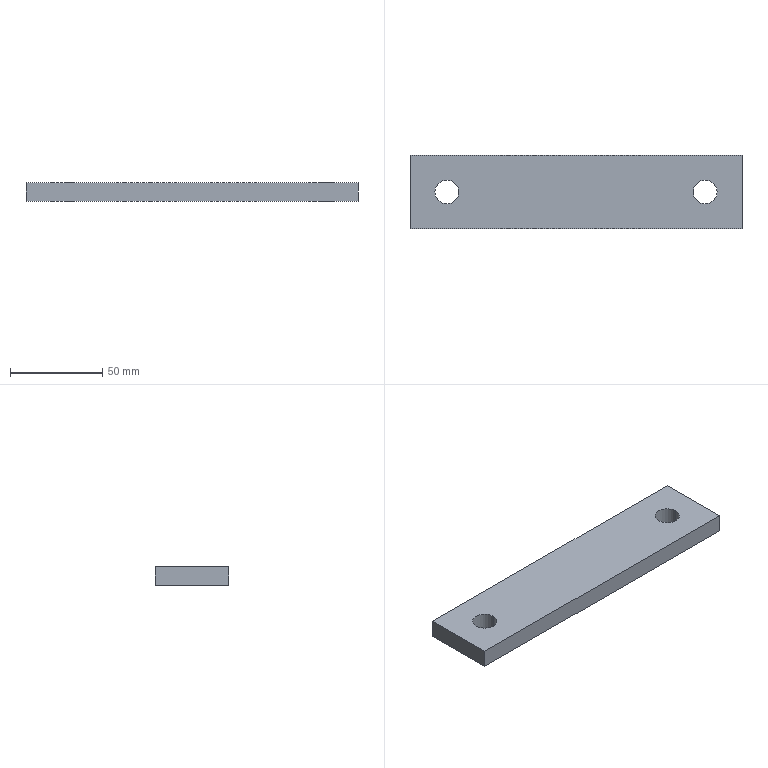Part | SolidWorks | features HoleWzd 2, Extrusion 1 | 1 solid | 10 faces | box 180 x 40 x 10 mm | volume 69345 mm3 | plane 6 | cylinder 4 | commonest cylinder face diameters 13 x4
STEP:
#1=CARTESIAN_POINT('',(-76.5,0.,-5.));
#2=VERTEX_POINT('',#1);
#3=CARTESIAN_POINT('',(-63.5,0.,-5.));
#4=VERTEX_POINT('',#3);
#5=CARTESIAN_POINT('',(-70.,0.,-5.));
#6=DIRECTION('',(0.,0.,1.));
#7=DIRECTION('',(1.,0.,0.));
#8=AXIS2_PLACEMENT_3D('',#5,#6,#7);
#9=CIRCLE('',#8,6.5);
#10=EDGE_CURVE('',#2,#4,#9,.T.);
#11=ORIENTED_EDGE('',*,*,#10,.F.);
#12=CARTESIAN_POINT('',(-76.5,0.,5.));
#13=VERTEX_POINT('',#12);
#14=CARTESIAN_POINT('',(-76.5,0.,5.));
#15=DIRECTION('',(0.,0.,1.));
#16=VECTOR('',#15,1000.);
#17=LINE('',#14,#16);
#18=EDGE_CURVE('',#2,#13,#17,.T.);
#19=ORIENTED_EDGE('',*,*,#18,.T.);
#20=CARTESIAN_POINT('',(-63.5,0.,5.));
#21=VERTEX_POINT('',#20);
#22=CARTESIAN_POINT('',(-70.,0.,5.));
#23=DIRECTION('',(0.,0.,1.));
#24=DIRECTION('',(1.,0.,0.));
#25=AXIS2_PLACEMENT_3D('',#22,#23,#24);
#26=CIRCLE('',#25,6.5);
#27=EDGE_CURVE('',#13,#21,#26,.T.);
#28=ORIENTED_EDGE('',*,*,#27,.T.);
#29=CARTESIAN_POINT('',(-63.5,0.,5.));
#30=DIRECTION('',(0.,0.,1.));
#31=VECTOR('',#30,1000.);
#32=LINE('',#29,#31);
#33=EDGE_CURVE('',#4,#21,#32,.T.);
#34=ORIENTED_EDGE('',*,*,#33,.F.);
#35=EDGE_LOOP('',(#11,#19,#28,#34));
#36=FACE_OUTER_BOUND('',#35,.T.);
#37=CARTESIAN_POINT('',(-70.,0.,5.));
#38=DIRECTION('',(0.,0.,1.));
#39=DIRECTION('',(1.,0.,0.));
#40=AXIS2_PLACEMENT_3D('',#37,#38,#39);
#41=CYLINDRICAL_SURFACE('',#40,6.5);
#42=ADVANCED_FACE('',(#36),#41,.F.);
#43=CARTESIAN_POINT('',(63.5,0.,-5.));
#44=VERTEX_POINT('',#43);
#45=CARTESIAN_POINT('',(76.5,0.,-5.));
#46=VERTEX_POINT('',#45);
#47=CARTESIAN_POINT('',(70.,0.,-5.));
#48=DIRECTION('',(0.,0.,1.));
#49=DIRECTION('',(1.,0.,0.));
#50=AXIS2_PLACEMENT_3D('',#47,#48,#49);
#51=CIRCLE('',#50,6.5);
#52=EDGE_CURVE('',#44,#46,#51,.T.);
#53=ORIENTED_EDGE('',*,*,#52,.F.);
#54=CARTESIAN_POINT('',(63.5,0.,5.));
#55=VERTEX_POINT('',#54);
#56=CARTESIAN_POINT('',(63.5,0.,5.));
#57=DIRECTION('',(0.,0.,1.));
#58=VECTOR('',#57,1000.);
#59=LINE('',#56,#58);
#60=EDGE_CURVE('',#44,#55,#59,.T.);
#61=ORIENTED_EDGE('',*,*,#60,.T.);
#62=CARTESIAN_POINT('',(76.5,0.,5.));
#63=VERTEX_POINT('',#62);
#64=CARTESIAN_POINT('',(70.,0.,5.));
#65=DIRECTION('',(0.,0.,1.));
#66=DIRECTION('',(1.,0.,0.));
#67=AXIS2_PLACEMENT_3D('',#64,#65,#66);
#68=CIRCLE('',#67,6.5);
#69=EDGE_CURVE('',#55,#63,#68,.T.);
#70=ORIENTED_EDGE('',*,*,#69,.T.);
#71=CARTESIAN_POINT('',(76.5,0.,5.));
#72=DIRECTION('',(0.,0.,1.));
#73=VECTOR('',#72,1000.);
#74=LINE('',#71,#73);
#75=EDGE_CURVE('',#46,#63,#74,.T.);
#76=ORIENTED_EDGE('',*,*,#75,.F.);
#77=EDGE_LOOP('',(#53,#61,#70,#76));
#78=FACE_OUTER_BOUND('',#77,.T.);
#79=CARTESIAN_POINT('',(70.,0.,5.));
#80=DIRECTION('',(0.,0.,1.));
#81=DIRECTION('',(1.,0.,0.));
#82=AXIS2_PLACEMENT_3D('',#79,#80,#81);
#83=CYLINDRICAL_SURFACE('',#82,6.5);
#84=ADVANCED_FACE('',(#78),#83,.F.);
#85=CARTESIAN_POINT('',(-90.,20.,-5.));
#86=VERTEX_POINT('',#85);
#87=CARTESIAN_POINT('',(-90.,-20.,-5.));
#88=VERTEX_POINT('',#87);
#89=CARTESIAN_POINT('',(-90.,-20.,-5.));
#90=DIRECTION('',(0.,-1.,0.));
#91=VECTOR('',#90,1000.);
#92=LINE('',#89,#91);
#93=EDGE_CURVE('',#86,#88,#92,.T.);
#94=ORIENTED_EDGE('',*,*,#93,.T.);
#95=CARTESIAN_POINT('',(-90.,-20.,5.));
#96=VERTEX_POINT('',#95);
#97=CARTESIAN_POINT('',(-90.,-20.,5.));
#98=DIRECTION('',(0.,0.,-1.));
#99=VECTOR('',#98,1000.);
#100=LINE('',#97,#99);
#101=EDGE_CURVE('',#96,#88,#100,.T.);
#102=ORIENTED_EDGE('',*,*,#101,.F.);
#103=CARTESIAN_POINT('',(-90.,20.,5.));
#104=VERTEX_POINT('',#103);
#105=CARTESIAN_POINT('',(-90.,-20.,5.));
#106=DIRECTION('',(0.,-1.,0.));
#107=VECTOR('',#106,1000.);
#108=LINE('',#105,#107);
#109=EDGE_CURVE('',#104,#96,#108,.T.);
#110=ORIENTED_EDGE('',*,*,#109,.F.);
#111=CARTESIAN_POINT('',(-90.,20.,5.));
#112=DIRECTION('',(0.,0.,-1.));
#113=VECTOR('',#112,1000.);
#114=LINE('',#111,#113);
#115=EDGE_CURVE('',#104,#86,#114,.T.);
#116=ORIENTED_EDGE('',*,*,#115,.T.);
#117=EDGE_LOOP('',(#94,#102,#110,#116));
#118=FACE_OUTER_BOUND('',#117,.T.);
#119=CARTESIAN_POINT('',(-90.,-20.,5.));
#120=DIRECTION('',(1.,0.,0.));
#121=DIRECTION('',(0.,0.,-1.));
#122=AXIS2_PLACEMENT_3D('',#119,#120,#121);
#123=PLANE('',#122);
#124=ADVANCED_FACE('',(#118),#123,.F.);
#125=CARTESIAN_POINT('',(90.,-20.,-5.));
#126=VERTEX_POINT('',#125);
#127=CARTESIAN_POINT('',(90.,-20.,-5.));
#128=DIRECTION('',(1.,0.,0.));
#129=VECTOR('',#128,1000.);
#130=LINE('',#127,#129);
#131=EDGE_CURVE('',#88,#126,#130,.T.);
#132=ORIENTED_EDGE('',*,*,#131,.T.);
#133=CARTESIAN_POINT('',(90.,-20.,5.));
#134=VERTEX_POINT('',#133);
#135=CARTESIAN_POINT('',(90.,-20.,5.));
#136=DIRECTION('',(0.,0.,-1.));
#137=VECTOR('',#136,1000.);
#138=LINE('',#135,#137);
#139=EDGE_CURVE('',#134,#126,#138,.T.);
#140=ORIENTED_EDGE('',*,*,#139,.F.);
#141=CARTESIAN_POINT('',(90.,-20.,5.));
#142=DIRECTION('',(1.,0.,0.));
#143=VECTOR('',#142,1000.);
#144=LINE('',#141,#143);
#145=EDGE_CURVE('',#96,#134,#144,.T.);
#146=ORIENTED_EDGE('',*,*,#145,.F.);
#147=ORIENTED_EDGE('',*,*,#101,.T.);
#148=EDGE_LOOP('',(#132,#140,#146,#147));
#149=FACE_OUTER_BOUND('',#148,.T.);
#150=CARTESIAN_POINT('',(90.,-20.,5.));
#151=DIRECTION('',(0.,1.,0.));
#152=DIRECTION('',(-1.,0.,0.));
#153=AXIS2_PLACEMENT_3D('',#150,#151,#152);
#154=PLANE('',#153);
#155=ADVANCED_FACE('',(#149),#154,.F.);
#156=CARTESIAN_POINT('',(90.,20.,-5.));
#157=VERTEX_POINT('',#156);
#158=CARTESIAN_POINT('',(90.,-20.,-5.));
#159=DIRECTION('',(0.,1.,0.));
#160=VECTOR('',#159,1000.);
#161=LINE('',#158,#160);
#162=EDGE_CURVE('',#126,#157,#161,.T.);
#163=ORIENTED_EDGE('',*,*,#162,.T.);
#164=CARTESIAN_POINT('',(90.,20.,5.));
#165=VERTEX_POINT('',#164);
#166=CARTESIAN_POINT('',(90.,20.,5.));
#167=DIRECTION('',(0.,0.,-1.));
#168=VECTOR('',#167,1000.);
#169=LINE('',#166,#168);
#170=EDGE_CURVE('',#165,#157,#169,.T.);
#171=ORIENTED_EDGE('',*,*,#170,.F.);
#172=CARTESIAN_POINT('',(90.,-20.,5.));
#173=DIRECTION('',(0.,1.,0.));
#174=VECTOR('',#173,1000.);
#175=LINE('',#172,#174);
#176=EDGE_CURVE('',#134,#165,#175,.T.);
#177=ORIENTED_EDGE('',*,*,#176,.F.);
#178=ORIENTED_EDGE('',*,*,#139,.T.);
#179=EDGE_LOOP('',(#163,#171,#177,#178));
#180=FACE_OUTER_BOUND('',#179,.T.);
#181=CARTESIAN_POINT('',(90.,-20.,5.));
#182=DIRECTION('',(-1.,0.,0.));
#183=DIRECTION('',(0.,0.,1.));
#184=AXIS2_PLACEMENT_3D('',#181,#182,#183);
#185=PLANE('',#184);
#186=ADVANCED_FACE('',(#180),#185,.F.);
#187=CARTESIAN_POINT('',(90.,20.,-5.));
#188=DIRECTION('',(-1.,0.,0.));
#189=VECTOR('',#188,1000.);
#190=LINE('',#187,#189);
#191=EDGE_CURVE('',#157,#86,#190,.T.);
#192=ORIENTED_EDGE('',*,*,#191,.T.);
#193=ORIENTED_EDGE('',*,*,#115,.F.);
#194=CARTESIAN_POINT('',(90.,20.,5.));
#195=DIRECTION('',(-1.,0.,0.));
#196=VECTOR('',#195,1000.);
#197=LINE('',#194,#196);
#198=EDGE_CURVE('',#165,#104,#197,.T.);
#199=ORIENTED_EDGE('',*,*,#198,.F.);
#200=ORIENTED_EDGE('',*,*,#170,.T.);
#201=EDGE_LOOP('',(#192,#193,#199,#200));
#202=FACE_OUTER_BOUND('',#201,.T.);
#203=CARTESIAN_POINT('',(90.,20.,5.));
#204=DIRECTION('',(0.,-1.,0.));
#205=DIRECTION('',(1.,0.,0.));
#206=AXIS2_PLACEMENT_3D('',#203,#204,#205);
#207=PLANE('',#206);
#208=ADVANCED_FACE('',(#202),#207,.F.);
#209=CARTESIAN_POINT('',(-70.,0.,5.));
#210=DIRECTION('',(0.,0.,1.));
#211=DIRECTION('',(1.,0.,0.));
#212=AXIS2_PLACEMENT_3D('',#209,#210,#211);
#213=CIRCLE('',#212,6.5);
#214=EDGE_CURVE('',#21,#13,#213,.T.);
#215=ORIENTED_EDGE('',*,*,#214,.F.);
#216=ORIENTED_EDGE('',*,*,#27,.F.);
#217=EDGE_LOOP('',(#215,#216));
#218=FACE_BOUND('',#217,.T.);
#219=CARTESIAN_POINT('',(70.,0.,5.));
#220=DIRECTION('',(0.,0.,1.));
#221=DIRECTION('',(1.,0.,0.));
#222=AXIS2_PLACEMENT_3D('',#219,#220,#221);
#223=CIRCLE('',#222,6.5);
#224=EDGE_CURVE('',#63,#55,#223,.T.);
#225=ORIENTED_EDGE('',*,*,#224,.F.);
#226=ORIENTED_EDGE('',*,*,#69,.F.);
#227=EDGE_LOOP('',(#225,#226));
#228=FACE_BOUND('',#227,.T.);
#229=ORIENTED_EDGE('',*,*,#109,.T.);
#230=ORIENTED_EDGE('',*,*,#145,.T.);
#231=ORIENTED_EDGE('',*,*,#176,.T.);
#232=ORIENTED_EDGE('',*,*,#198,.T.);
#233=EDGE_LOOP('',(#229,#230,#231,#232));
#234=FACE_OUTER_BOUND('',#233,.T.);
#235=CARTESIAN_POINT('',(0.,0.,5.));
#236=DIRECTION('',(0.,0.,1.));
#237=DIRECTION('',(1.,0.,0.));
#238=AXIS2_PLACEMENT_3D('',#235,#236,#237);
#239=PLANE('',#238);
#240=ADVANCED_FACE('',(#218,#228,#234),#239,.T.);
#241=CARTESIAN_POINT('',(-70.,0.,-5.));
#242=DIRECTION('',(0.,0.,1.));
#243=DIRECTION('',(1.,0.,0.));
#244=AXIS2_PLACEMENT_3D('',#241,#242,#243);
#245=CIRCLE('',#244,6.5);
#246=EDGE_CURVE('',#4,#2,#245,.T.);
#247=ORIENTED_EDGE('',*,*,#246,.T.);
#248=ORIENTED_EDGE('',*,*,#10,.T.);
#249=EDGE_LOOP('',(#247,#248));
#250=FACE_BOUND('',#249,.T.);
#251=CARTESIAN_POINT('',(70.,0.,-5.));
#252=DIRECTION('',(0.,0.,1.));
#253=DIRECTION('',(1.,0.,0.));
#254=AXIS2_PLACEMENT_3D('',#251,#252,#253);
#255=CIRCLE('',#254,6.5);
#256=EDGE_CURVE('',#46,#44,#255,.T.);
#257=ORIENTED_EDGE('',*,*,#256,.T.);
#258=ORIENTED_EDGE('',*,*,#52,.T.);
#259=EDGE_LOOP('',(#257,#258));
#260=FACE_BOUND('',#259,.T.);
#261=ORIENTED_EDGE('',*,*,#93,.F.);
#262=ORIENTED_EDGE('',*,*,#191,.F.);
#263=ORIENTED_EDGE('',*,*,#162,.F.);
#264=ORIENTED_EDGE('',*,*,#131,.F.);
#265=EDGE_LOOP('',(#261,#262,#263,#264));
#266=FACE_OUTER_BOUND('',#265,.T.);
#267=CARTESIAN_POINT('',(0.,0.,-5.));
#268=DIRECTION('',(0.,0.,1.));
#269=DIRECTION('',(1.,0.,0.));
#270=AXIS2_PLACEMENT_3D('',#267,#268,#269);
#271=PLANE('',#270);
#272=ADVANCED_FACE('',(#250,#260,#266),#271,.F.);
#273=ORIENTED_EDGE('',*,*,#60,.F.);
#274=ORIENTED_EDGE('',*,*,#256,.F.);
#275=ORIENTED_EDGE('',*,*,#75,.T.);
#276=ORIENTED_EDGE('',*,*,#224,.T.);
#277=EDGE_LOOP('',(#273,#274,#275,#276));
#278=FACE_OUTER_BOUND('',#277,.T.);
#279=CARTESIAN_POINT('',(70.,0.,5.));
#280=DIRECTION('',(0.,0.,1.));
#281=DIRECTION('',(1.,0.,0.));
#282=AXIS2_PLACEMENT_3D('',#279,#280,#281);
#283=CYLINDRICAL_SURFACE('',#282,6.5);
#284=ADVANCED_FACE('',(#278),#283,.F.);
#285=ORIENTED_EDGE('',*,*,#18,.F.);
#286=ORIENTED_EDGE('',*,*,#246,.F.);
#287=ORIENTED_EDGE('',*,*,#33,.T.);
#288=ORIENTED_EDGE('',*,*,#214,.T.);
#289=EDGE_LOOP('',(#285,#286,#287,#288));
#290=FACE_OUTER_BOUND('',#289,.T.);
#291=CARTESIAN_POINT('',(-70.,0.,5.));
#292=DIRECTION('',(0.,0.,1.));
#293=DIRECTION('',(1.,0.,0.));
#294=AXIS2_PLACEMENT_3D('',#291,#292,#293);
#295=CYLINDRICAL_SURFACE('',#294,6.5);
#296=ADVANCED_FACE('',(#290),#295,.F.);
#297=CLOSED_SHELL('',(#42,#84,#124,#155,#186,#208,#240,#272,#284,#296));
#298=MANIFOLD_SOLID_BREP('',#297);
#299=CARTESIAN_POINT('',(0.,0.,0.));
#300=DIRECTION('',(0.,0.,1.));
#301=DIRECTION('',(1.,0.,0.));
#302=AXIS2_PLACEMENT_3D('',#299,#300,#301);
#303=(LENGTH_UNIT()NAMED_UNIT(*)SI_UNIT(.MILLI.,.METRE.));
#304=UNCERTAINTY_MEASURE_WITH_UNIT(LENGTH_MEASURE(0.00001),#303,'','');
#305=(NAMED_UNIT(*)PLANE_ANGLE_UNIT()SI_UNIT($,.RADIAN.));
#306=(NAMED_UNIT(*)SI_UNIT($,.STERADIAN.)SOLID_ANGLE_UNIT());
#307=(GEOMETRIC_REPRESENTATION_CONTEXT(3)GLOBAL_UNCERTAINTY_ASSIGNED_CONTEXT((#304))GLOBAL_UNIT_ASSIGNED_CONTEXT((#303,#305,#306))REPRESENTATION_CONTEXT('',''));
#308=ADVANCED_BREP_SHAPE_REPRESENTATION('',(#298,#302),#307);